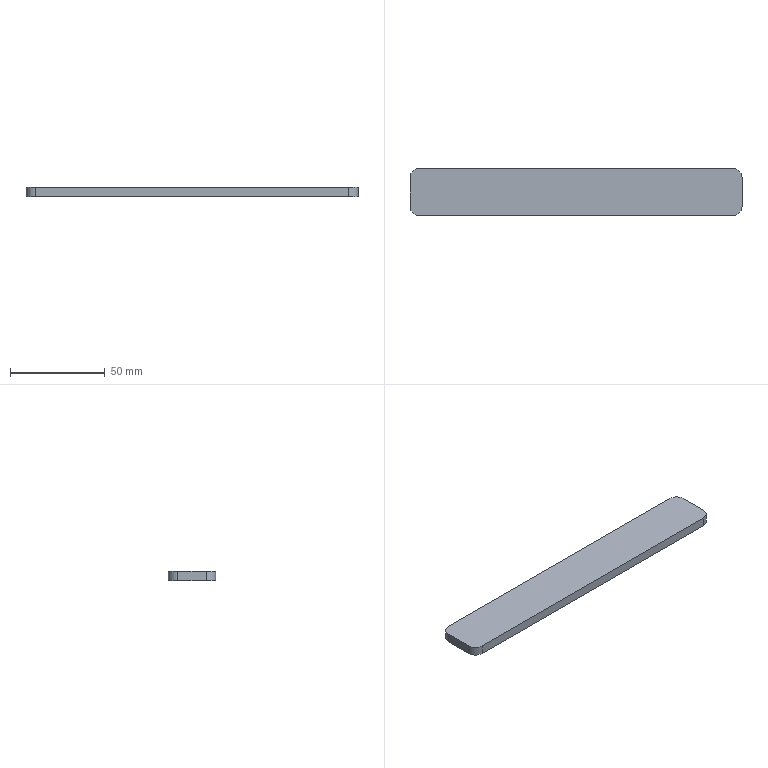Part | NX | features BREP 1 | 1 solid | 10 faces | box 175 x 25 x 5 mm | volume 21768 mm3 | plane 6 | cylinder 4 | commonest cylinder face diameters 10 x4
STEP:
#1=CARTESIAN_POINT('',(87.5,7.5,0.));
#2=VERTEX_POINT('',#1);
#3=CARTESIAN_POINT('',(82.5,12.5,0.));
#4=VERTEX_POINT('',#3);
#5=CARTESIAN_POINT('',(82.5,7.5,0.));
#6=DIRECTION('',(0.,0.,1.));
#7=DIRECTION('',(-1.,0.,0.));
#8=AXIS2_PLACEMENT_3D('',#5,#6,#7);
#9=CIRCLE('',#8,5.);
#10=EDGE_CURVE('',#2,#4,#9,.T.);
#11=ORIENTED_EDGE('',*,*,#10,.T.);
#12=CARTESIAN_POINT('',(82.5,12.5,5.));
#13=VERTEX_POINT('',#12);
#14=CARTESIAN_POINT('',(82.5,12.5,5.));
#15=DIRECTION('',(0.,0.,-1.));
#16=VECTOR('',#15,1000.);
#17=LINE('',#14,#16);
#18=EDGE_CURVE('',#13,#4,#17,.T.);
#19=ORIENTED_EDGE('',*,*,#18,.F.);
#20=CARTESIAN_POINT('',(87.5,7.5,5.));
#21=VERTEX_POINT('',#20);
#22=CARTESIAN_POINT('',(82.5,7.5,5.));
#23=DIRECTION('',(0.,0.,1.));
#24=DIRECTION('',(-1.,0.,0.));
#25=AXIS2_PLACEMENT_3D('',#22,#23,#24);
#26=CIRCLE('',#25,5.);
#27=EDGE_CURVE('',#21,#13,#26,.T.);
#28=ORIENTED_EDGE('',*,*,#27,.F.);
#29=CARTESIAN_POINT('',(87.5,7.5,5.));
#30=DIRECTION('',(0.,0.,-1.));
#31=VECTOR('',#30,1000.);
#32=LINE('',#29,#31);
#33=EDGE_CURVE('',#21,#2,#32,.T.);
#34=ORIENTED_EDGE('',*,*,#33,.T.);
#35=EDGE_LOOP('',(#11,#19,#28,#34));
#36=FACE_BOUND('',#35,.T.);
#37=CARTESIAN_POINT('',(82.5,7.5,5.));
#38=DIRECTION('',(0.,0.,-1.));
#39=DIRECTION('',(-1.,0.,0.));
#40=AXIS2_PLACEMENT_3D('',#37,#38,#39);
#41=CYLINDRICAL_SURFACE('',#40,5.);
#42=ADVANCED_FACE('',(#36),#41,.T.);
#43=CARTESIAN_POINT('',(-82.5,12.5,0.));
#44=VERTEX_POINT('',#43);
#45=CARTESIAN_POINT('',(-82.5,12.5,0.));
#46=DIRECTION('',(-1.,0.,0.));
#47=VECTOR('',#46,1000.);
#48=LINE('',#45,#47);
#49=EDGE_CURVE('',#4,#44,#48,.T.);
#50=ORIENTED_EDGE('',*,*,#49,.T.);
#51=CARTESIAN_POINT('',(-82.5,12.5,5.));
#52=VERTEX_POINT('',#51);
#53=CARTESIAN_POINT('',(-82.5,12.5,5.));
#54=DIRECTION('',(0.,0.,-1.));
#55=VECTOR('',#54,1000.);
#56=LINE('',#53,#55);
#57=EDGE_CURVE('',#52,#44,#56,.T.);
#58=ORIENTED_EDGE('',*,*,#57,.F.);
#59=CARTESIAN_POINT('',(-82.5,12.5,5.));
#60=DIRECTION('',(-1.,0.,0.));
#61=VECTOR('',#60,1000.);
#62=LINE('',#59,#61);
#63=EDGE_CURVE('',#13,#52,#62,.T.);
#64=ORIENTED_EDGE('',*,*,#63,.F.);
#65=ORIENTED_EDGE('',*,*,#18,.T.);
#66=EDGE_LOOP('',(#50,#58,#64,#65));
#67=FACE_BOUND('',#66,.T.);
#68=CARTESIAN_POINT('',(-82.5,12.5,5.));
#69=DIRECTION('',(0.,-1.,0.));
#70=DIRECTION('',(0.,0.,-1.));
#71=AXIS2_PLACEMENT_3D('',#68,#69,#70);
#72=PLANE('',#71);
#73=ADVANCED_FACE('',(#67),#72,.F.);
#74=CARTESIAN_POINT('',(-87.5,7.5,0.));
#75=VERTEX_POINT('',#74);
#76=CARTESIAN_POINT('',(-82.5,7.5,0.));
#77=DIRECTION('',(0.,0.,1.));
#78=DIRECTION('',(1.,0.,0.));
#79=AXIS2_PLACEMENT_3D('',#76,#77,#78);
#80=CIRCLE('',#79,5.);
#81=EDGE_CURVE('',#44,#75,#80,.T.);
#82=ORIENTED_EDGE('',*,*,#81,.T.);
#83=CARTESIAN_POINT('',(-87.5,7.5,5.));
#84=VERTEX_POINT('',#83);
#85=CARTESIAN_POINT('',(-87.5,7.5,5.));
#86=DIRECTION('',(0.,0.,-1.));
#87=VECTOR('',#86,1000.);
#88=LINE('',#85,#87);
#89=EDGE_CURVE('',#84,#75,#88,.T.);
#90=ORIENTED_EDGE('',*,*,#89,.F.);
#91=CARTESIAN_POINT('',(-82.5,7.5,5.));
#92=DIRECTION('',(0.,0.,1.));
#93=DIRECTION('',(1.,0.,0.));
#94=AXIS2_PLACEMENT_3D('',#91,#92,#93);
#95=CIRCLE('',#94,5.);
#96=EDGE_CURVE('',#52,#84,#95,.T.);
#97=ORIENTED_EDGE('',*,*,#96,.F.);
#98=ORIENTED_EDGE('',*,*,#57,.T.);
#99=EDGE_LOOP('',(#82,#90,#97,#98));
#100=FACE_BOUND('',#99,.T.);
#101=CARTESIAN_POINT('',(-82.5,7.5,5.));
#102=DIRECTION('',(0.,0.,-1.));
#103=DIRECTION('',(-1.,0.,0.));
#104=AXIS2_PLACEMENT_3D('',#101,#102,#103);
#105=CYLINDRICAL_SURFACE('',#104,5.);
#106=ADVANCED_FACE('',(#100),#105,.T.);
#107=CARTESIAN_POINT('',(-87.5,-7.5,0.));
#108=VERTEX_POINT('',#107);
#109=CARTESIAN_POINT('',(-87.5,7.5,0.));
#110=DIRECTION('',(0.,-1.,0.));
#111=VECTOR('',#110,1000.);
#112=LINE('',#109,#111);
#113=EDGE_CURVE('',#75,#108,#112,.T.);
#114=ORIENTED_EDGE('',*,*,#113,.T.);
#115=CARTESIAN_POINT('',(-87.5,-7.5,5.));
#116=VERTEX_POINT('',#115);
#117=CARTESIAN_POINT('',(-87.5,-7.5,5.));
#118=DIRECTION('',(0.,0.,-1.));
#119=VECTOR('',#118,1000.);
#120=LINE('',#117,#119);
#121=EDGE_CURVE('',#116,#108,#120,.T.);
#122=ORIENTED_EDGE('',*,*,#121,.F.);
#123=CARTESIAN_POINT('',(-87.5,7.5,5.));
#124=DIRECTION('',(0.,-1.,0.));
#125=VECTOR('',#124,1000.);
#126=LINE('',#123,#125);
#127=EDGE_CURVE('',#84,#116,#126,.T.);
#128=ORIENTED_EDGE('',*,*,#127,.F.);
#129=ORIENTED_EDGE('',*,*,#89,.T.);
#130=EDGE_LOOP('',(#114,#122,#128,#129));
#131=FACE_BOUND('',#130,.T.);
#132=CARTESIAN_POINT('',(-87.5,7.5,5.));
#133=DIRECTION('',(1.,0.,0.));
#134=DIRECTION('',(0.,1.,0.));
#135=AXIS2_PLACEMENT_3D('',#132,#133,#134);
#136=PLANE('',#135);
#137=ADVANCED_FACE('',(#131),#136,.F.);
#138=CARTESIAN_POINT('',(-82.5,-12.5,0.));
#139=VERTEX_POINT('',#138);
#140=CARTESIAN_POINT('',(-82.5,-7.5,0.));
#141=DIRECTION('',(0.,0.,1.));
#142=DIRECTION('',(1.,0.,0.));
#143=AXIS2_PLACEMENT_3D('',#140,#141,#142);
#144=CIRCLE('',#143,5.);
#145=EDGE_CURVE('',#108,#139,#144,.T.);
#146=ORIENTED_EDGE('',*,*,#145,.T.);
#147=CARTESIAN_POINT('',(-82.5,-12.5,5.));
#148=VERTEX_POINT('',#147);
#149=CARTESIAN_POINT('',(-82.5,-12.5,5.));
#150=DIRECTION('',(0.,0.,-1.));
#151=VECTOR('',#150,1000.);
#152=LINE('',#149,#151);
#153=EDGE_CURVE('',#148,#139,#152,.T.);
#154=ORIENTED_EDGE('',*,*,#153,.F.);
#155=CARTESIAN_POINT('',(-82.5,-7.5,5.));
#156=DIRECTION('',(0.,0.,1.));
#157=DIRECTION('',(1.,0.,0.));
#158=AXIS2_PLACEMENT_3D('',#155,#156,#157);
#159=CIRCLE('',#158,5.);
#160=EDGE_CURVE('',#116,#148,#159,.T.);
#161=ORIENTED_EDGE('',*,*,#160,.F.);
#162=ORIENTED_EDGE('',*,*,#121,.T.);
#163=EDGE_LOOP('',(#146,#154,#161,#162));
#164=FACE_BOUND('',#163,.T.);
#165=CARTESIAN_POINT('',(-82.5,-7.5,5.));
#166=DIRECTION('',(0.,0.,-1.));
#167=DIRECTION('',(-1.,0.,0.));
#168=AXIS2_PLACEMENT_3D('',#165,#166,#167);
#169=CYLINDRICAL_SURFACE('',#168,5.);
#170=ADVANCED_FACE('',(#164),#169,.T.);
#171=CARTESIAN_POINT('',(82.5,-12.5,0.));
#172=VERTEX_POINT('',#171);
#173=CARTESIAN_POINT('',(-82.5,-12.5,0.));
#174=DIRECTION('',(1.,0.,0.));
#175=VECTOR('',#174,1000.);
#176=LINE('',#173,#175);
#177=EDGE_CURVE('',#139,#172,#176,.T.);
#178=ORIENTED_EDGE('',*,*,#177,.T.);
#179=CARTESIAN_POINT('',(82.5,-12.5,5.));
#180=VERTEX_POINT('',#179);
#181=CARTESIAN_POINT('',(82.5,-12.5,5.));
#182=DIRECTION('',(0.,0.,-1.));
#183=VECTOR('',#182,1000.);
#184=LINE('',#181,#183);
#185=EDGE_CURVE('',#180,#172,#184,.T.);
#186=ORIENTED_EDGE('',*,*,#185,.F.);
#187=CARTESIAN_POINT('',(-82.5,-12.5,5.));
#188=DIRECTION('',(1.,0.,0.));
#189=VECTOR('',#188,1000.);
#190=LINE('',#187,#189);
#191=EDGE_CURVE('',#148,#180,#190,.T.);
#192=ORIENTED_EDGE('',*,*,#191,.F.);
#193=ORIENTED_EDGE('',*,*,#153,.T.);
#194=EDGE_LOOP('',(#178,#186,#192,#193));
#195=FACE_BOUND('',#194,.T.);
#196=CARTESIAN_POINT('',(-82.5,-12.5,5.));
#197=DIRECTION('',(0.,1.,0.));
#198=DIRECTION('',(1.,0.,0.));
#199=AXIS2_PLACEMENT_3D('',#196,#197,#198);
#200=PLANE('',#199);
#201=ADVANCED_FACE('',(#195),#200,.F.);
#202=CARTESIAN_POINT('',(87.5,-7.5,0.));
#203=VERTEX_POINT('',#202);
#204=CARTESIAN_POINT('',(82.5,-7.5,0.));
#205=DIRECTION('',(0.,0.,1.));
#206=DIRECTION('',(1.,0.,0.));
#207=AXIS2_PLACEMENT_3D('',#204,#205,#206);
#208=CIRCLE('',#207,5.);
#209=EDGE_CURVE('',#172,#203,#208,.T.);
#210=ORIENTED_EDGE('',*,*,#209,.T.);
#211=CARTESIAN_POINT('',(87.5,-7.5,5.));
#212=VERTEX_POINT('',#211);
#213=CARTESIAN_POINT('',(87.5,-7.5,5.));
#214=DIRECTION('',(0.,0.,-1.));
#215=VECTOR('',#214,1000.);
#216=LINE('',#213,#215);
#217=EDGE_CURVE('',#212,#203,#216,.T.);
#218=ORIENTED_EDGE('',*,*,#217,.F.);
#219=CARTESIAN_POINT('',(82.5,-7.5,5.));
#220=DIRECTION('',(0.,0.,1.));
#221=DIRECTION('',(1.,0.,0.));
#222=AXIS2_PLACEMENT_3D('',#219,#220,#221);
#223=CIRCLE('',#222,5.);
#224=EDGE_CURVE('',#180,#212,#223,.T.);
#225=ORIENTED_EDGE('',*,*,#224,.F.);
#226=ORIENTED_EDGE('',*,*,#185,.T.);
#227=EDGE_LOOP('',(#210,#218,#225,#226));
#228=FACE_BOUND('',#227,.T.);
#229=CARTESIAN_POINT('',(82.5,-7.5,5.));
#230=DIRECTION('',(0.,0.,-1.));
#231=DIRECTION('',(-1.,0.,0.));
#232=AXIS2_PLACEMENT_3D('',#229,#230,#231);
#233=CYLINDRICAL_SURFACE('',#232,5.);
#234=ADVANCED_FACE('',(#228),#233,.T.);
#235=CARTESIAN_POINT('',(87.5,7.5,0.));
#236=DIRECTION('',(0.,1.,0.));
#237=VECTOR('',#236,1000.);
#238=LINE('',#235,#237);
#239=EDGE_CURVE('',#203,#2,#238,.T.);
#240=ORIENTED_EDGE('',*,*,#239,.T.);
#241=ORIENTED_EDGE('',*,*,#33,.F.);
#242=CARTESIAN_POINT('',(87.5,7.5,5.));
#243=DIRECTION('',(0.,1.,0.));
#244=VECTOR('',#243,1000.);
#245=LINE('',#242,#244);
#246=EDGE_CURVE('',#212,#21,#245,.T.);
#247=ORIENTED_EDGE('',*,*,#246,.F.);
#248=ORIENTED_EDGE('',*,*,#217,.T.);
#249=EDGE_LOOP('',(#240,#241,#247,#248));
#250=FACE_BOUND('',#249,.T.);
#251=CARTESIAN_POINT('',(87.5,7.5,5.));
#252=DIRECTION('',(-1.,0.,0.));
#253=DIRECTION('',(0.,0.,1.));
#254=AXIS2_PLACEMENT_3D('',#251,#252,#253);
#255=PLANE('',#254);
#256=ADVANCED_FACE('',(#250),#255,.F.);
#257=ORIENTED_EDGE('',*,*,#27,.T.);
#258=ORIENTED_EDGE('',*,*,#63,.T.);
#259=ORIENTED_EDGE('',*,*,#96,.T.);
#260=ORIENTED_EDGE('',*,*,#127,.T.);
#261=ORIENTED_EDGE('',*,*,#160,.T.);
#262=ORIENTED_EDGE('',*,*,#191,.T.);
#263=ORIENTED_EDGE('',*,*,#224,.T.);
#264=ORIENTED_EDGE('',*,*,#246,.T.);
#265=EDGE_LOOP('',(#257,#258,#259,#260,#261,#262,#263,#264));
#266=FACE_BOUND('',#265,.T.);
#267=CARTESIAN_POINT('',(82.5,7.5,5.));
#268=DIRECTION('',(0.,0.,-1.));
#269=DIRECTION('',(0.,-1.,0.));
#270=AXIS2_PLACEMENT_3D('',#267,#268,#269);
#271=PLANE('',#270);
#272=ADVANCED_FACE('',(#266),#271,.F.);
#273=ORIENTED_EDGE('',*,*,#10,.F.);
#274=ORIENTED_EDGE('',*,*,#239,.F.);
#275=ORIENTED_EDGE('',*,*,#209,.F.);
#276=ORIENTED_EDGE('',*,*,#177,.F.);
#277=ORIENTED_EDGE('',*,*,#145,.F.);
#278=ORIENTED_EDGE('',*,*,#113,.F.);
#279=ORIENTED_EDGE('',*,*,#81,.F.);
#280=ORIENTED_EDGE('',*,*,#49,.F.);
#281=EDGE_LOOP('',(#273,#274,#275,#276,#277,#278,#279,#280));
#282=FACE_BOUND('',#281,.T.);
#283=CARTESIAN_POINT('',(82.5,7.5,0.));
#284=DIRECTION('',(0.,0.,-1.));
#285=DIRECTION('',(0.,-1.,0.));
#286=AXIS2_PLACEMENT_3D('',#283,#284,#285);
#287=PLANE('',#286);
#288=ADVANCED_FACE('',(#282),#287,.T.);
#289=CLOSED_SHELL('',(#42,#73,#106,#137,#170,#201,#234,#256,#272,#288));
#290=MANIFOLD_SOLID_BREP('',#289);
#291=(LENGTH_UNIT()NAMED_UNIT(*)SI_UNIT(.MILLI.,.METRE.));
#292=UNCERTAINTY_MEASURE_WITH_UNIT(LENGTH_MEASURE(0.00001),#291,'','');
#293=(NAMED_UNIT(*)PLANE_ANGLE_UNIT()SI_UNIT($,.RADIAN.));
#294=(NAMED_UNIT(*)SI_UNIT($,.STERADIAN.)SOLID_ANGLE_UNIT());
#295=(GEOMETRIC_REPRESENTATION_CONTEXT(3)GLOBAL_UNCERTAINTY_ASSIGNED_CONTEXT((#292))GLOBAL_UNIT_ASSIGNED_CONTEXT((#291,#293,#294))REPRESENTATION_CONTEXT('',''));
#296=ADVANCED_BREP_SHAPE_REPRESENTATION('',(#290),#295);